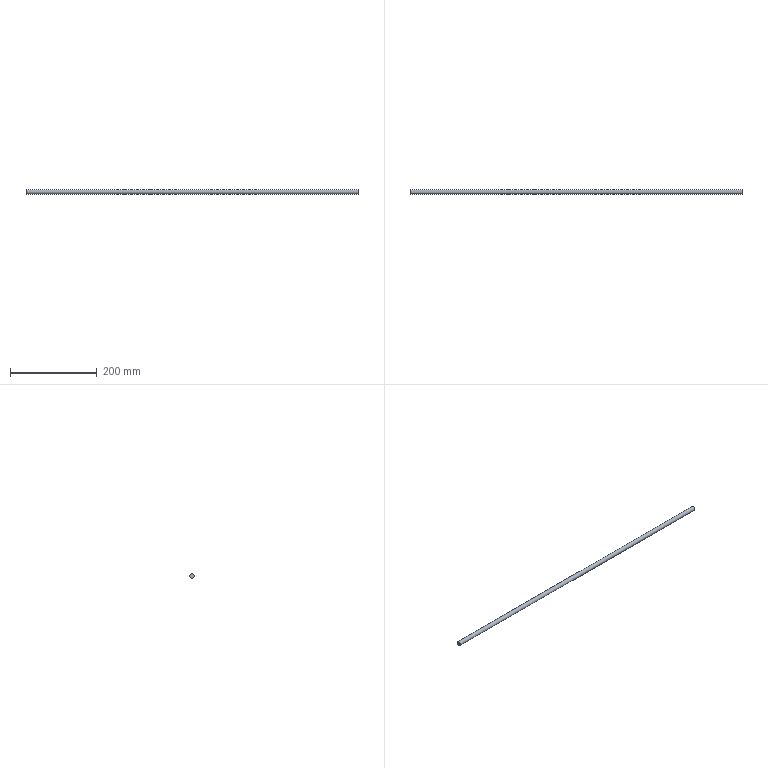Part | NX | features solid 2 | 1 solid | 3 faces | box 764 x 10 x 10 mm | volume 60004 mm3 | plane 2 | cylinder 1 | commonest cylinder face diameters 10 x1
STEP:
#1=CARTESIAN_POINT('',(411.,-337.5,-177.));
#2=VERTEX_POINT('',#1);
#3=CARTESIAN_POINT('',(411.,-337.5,-172.));
#4=DIRECTION('',(1.,0.,0.));
#5=DIRECTION('',(0.,0.,-1.));
#6=AXIS2_PLACEMENT_3D('',#3,#4,#5);
#7=CIRCLE('',#6,5.);
#8=EDGE_CURVE('',#2,#2,#7,.F.);
#9=ORIENTED_EDGE('',*,*,#8,.T.);
#10=EDGE_LOOP('',(#9));
#11=FACE_BOUND('',#10,.T.);
#12=CARTESIAN_POINT('',(411.,-337.5,-172.));
#13=DIRECTION('',(1.,0.,0.));
#14=DIRECTION('',(0.,0.,1.));
#15=AXIS2_PLACEMENT_3D('',#12,#13,#14);
#16=PLANE('',#15);
#17=ADVANCED_FACE('',(#11),#16,.F.);
#18=CARTESIAN_POINT('',(1175.,-337.5,-177.));
#19=VERTEX_POINT('',#18);
#20=CARTESIAN_POINT('',(1175.,-337.5,-172.));
#21=DIRECTION('',(1.,0.,0.));
#22=DIRECTION('',(0.,0.,-1.));
#23=AXIS2_PLACEMENT_3D('',#20,#21,#22);
#24=CIRCLE('',#23,5.);
#25=EDGE_CURVE('',#19,#19,#24,.T.);
#26=ORIENTED_EDGE('',*,*,#25,.F.);
#27=EDGE_LOOP('',(#26));
#28=FACE_BOUND('',#27,.T.);
#29=ORIENTED_EDGE('',*,*,#8,.F.);
#30=EDGE_LOOP('',(#29));
#31=FACE_BOUND('',#30,.T.);
#32=CARTESIAN_POINT('',(1611.,-337.5,-172.));
#33=DIRECTION('',(-1.,0.,0.));
#34=DIRECTION('',(0.,0.,-1.));
#35=AXIS2_PLACEMENT_3D('',#32,#33,#34);
#36=CYLINDRICAL_SURFACE('',#35,5.);
#37=ADVANCED_FACE('',(#28,#31),#36,.T.);
#38=ORIENTED_EDGE('',*,*,#25,.T.);
#39=EDGE_LOOP('',(#38));
#40=FACE_BOUND('',#39,.T.);
#41=CARTESIAN_POINT('',(1175.,-240.,-260.));
#42=DIRECTION('',(1.,0.,0.));
#43=DIRECTION('',(0.,0.,1.));
#44=AXIS2_PLACEMENT_3D('',#41,#42,#43);
#45=PLANE('',#44);
#46=ADVANCED_FACE('',(#40),#45,.T.);
#47=CLOSED_SHELL('',(#17,#37,#46));
#48=MANIFOLD_SOLID_BREP('',#47);
#49=(LENGTH_UNIT()NAMED_UNIT(*)SI_UNIT(.MILLI.,.METRE.));
#50=UNCERTAINTY_MEASURE_WITH_UNIT(LENGTH_MEASURE(0.00001),#49,'','');
#51=(NAMED_UNIT(*)PLANE_ANGLE_UNIT()SI_UNIT($,.RADIAN.));
#52=(NAMED_UNIT(*)SI_UNIT($,.STERADIAN.)SOLID_ANGLE_UNIT());
#53=(GEOMETRIC_REPRESENTATION_CONTEXT(3)GLOBAL_UNCERTAINTY_ASSIGNED_CONTEXT((#50))GLOBAL_UNIT_ASSIGNED_CONTEXT((#49,#51,#52))REPRESENTATION_CONTEXT('',''));
#54=ADVANCED_BREP_SHAPE_REPRESENTATION('',(#48),#53);